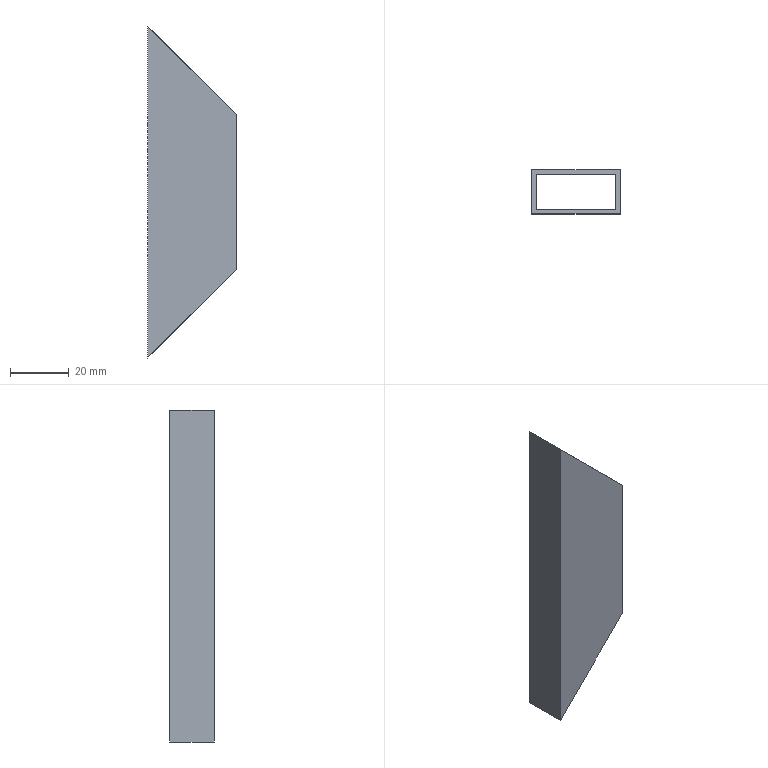Part | STEP file | Q7C0110 | 1 solid | 10 faces | box 30 x 15 x 113 mm | volume 10458 mm3 | plane 10
STEP:
#1=CARTESIAN_POINT('',(0.,0.,0.));
#2=DIRECTION('',(0.,0.,1.));
#3=DIRECTION('',(1.,0.,0.));
#4=AXIS2_PLACEMENT_3D('',#1,#2,#3);
#5=CARTESIAN_POINT('',(15.,7.5,83.));
#6=VERTEX_POINT('',#5);
#7=CARTESIAN_POINT('',(15.,7.5,30.));
#8=VERTEX_POINT('',#7);
#9=CARTESIAN_POINT('',(15.,7.5,150.));
#10=DIRECTION('',(0.,0.,-1.));
#11=VECTOR('',#10,1.);
#12=LINE('',#9,#11);
#13=CARTESIAN_POINT('',(15.,7.5,150.));
#14=DIRECTION('',(-1.,0.,0.));
#15=DIRECTION('',(0.,0.,1.));
#16=AXIS2_PLACEMENT_3D('',#13,#14,#15);
#17=PLANE('',#16);
#18=CARTESIAN_POINT('',(0.,0.));
#19=DIRECTION('',(-1.,0.));
#20=VECTOR('',#19,1.);
#21=LINE('',#18,#20);
#22=(GEOMETRIC_REPRESENTATION_CONTEXT(2)PARAMETRIC_REPRESENTATION_CONTEXT()REPRESENTATION_CONTEXT('',''));
#23=DEFINITIONAL_REPRESENTATION('',(#21),#22);
#24=PCURVE('',#17,#23);
#25=CARTESIAN_POINT('',(-15.,7.5,150.));
#26=DIRECTION('',(0.,-1.,0.));
#27=DIRECTION('',(0.,0.,-1.));
#28=AXIS2_PLACEMENT_3D('',#25,#26,#27);
#29=PLANE('',#28);
#30=CARTESIAN_POINT('',(0.,30.));
#31=DIRECTION('',(1.,0.));
#32=VECTOR('',#31,1.);
#33=LINE('',#30,#32);
#34=(GEOMETRIC_REPRESENTATION_CONTEXT(2)PARAMETRIC_REPRESENTATION_CONTEXT()REPRESENTATION_CONTEXT('',''));
#35=DEFINITIONAL_REPRESENTATION('',(#33),#34);
#36=PCURVE('',#29,#35);
#37=SURFACE_CURVE('',#12,(#24,#36),.PCURVE_S1.);
#38=EDGE_CURVE('',#6,#8,#37,.T.);
#39=ORIENTED_EDGE('',*,*,#38,.F.);
#40=CARTESIAN_POINT('',(15.,-7.5,83.));
#41=VERTEX_POINT('',#40);
#42=CARTESIAN_POINT('',(15.,-7.5,83.));
#43=DIRECTION('',(0.,1.,0.));
#44=VECTOR('',#43,1.);
#45=LINE('',#42,#44);
#46=CARTESIAN_POINT('',(-67.,-15.));
#47=DIRECTION('',(0.,1.));
#48=VECTOR('',#47,1.);
#49=LINE('',#46,#48);
#50=(GEOMETRIC_REPRESENTATION_CONTEXT(2)PARAMETRIC_REPRESENTATION_CONTEXT()REPRESENTATION_CONTEXT('',''));
#51=DEFINITIONAL_REPRESENTATION('',(#49),#50);
#52=PCURVE('',#17,#51);
#53=CARTESIAN_POINT('',(15.,-7.5,83.));
#54=DIRECTION('',(-0.7071,0.,-0.7071));
#55=DIRECTION('',(-0.7071,0.,0.7071));
#56=AXIS2_PLACEMENT_3D('',#53,#54,#55);
#57=PLANE('',#56);
#58=CARTESIAN_POINT('',(0.,0.));
#59=DIRECTION('',(0.,1.));
#60=VECTOR('',#59,1.);
#61=LINE('',#58,#60);
#62=(GEOMETRIC_REPRESENTATION_CONTEXT(2)PARAMETRIC_REPRESENTATION_CONTEXT()REPRESENTATION_CONTEXT('',''));
#63=DEFINITIONAL_REPRESENTATION('',(#61),#62);
#64=PCURVE('',#57,#63);
#65=SURFACE_CURVE('',#45,(#52,#64),.PCURVE_S1.);
#66=EDGE_CURVE('',#41,#6,#65,.T.);
#67=ORIENTED_EDGE('',*,*,#66,.F.);
#68=CARTESIAN_POINT('',(15.,-7.5,30.));
#69=VERTEX_POINT('',#68);
#70=CARTESIAN_POINT('',(15.,-7.5,150.));
#71=DIRECTION('',(0.,0.,-1.));
#72=VECTOR('',#71,1.);
#73=LINE('',#70,#72);
#74=CARTESIAN_POINT('',(0.,-15.));
#75=DIRECTION('',(-1.,0.));
#76=VECTOR('',#75,1.);
#77=LINE('',#74,#76);
#78=(GEOMETRIC_REPRESENTATION_CONTEXT(2)PARAMETRIC_REPRESENTATION_CONTEXT()REPRESENTATION_CONTEXT('',''));
#79=DEFINITIONAL_REPRESENTATION('',(#77),#78);
#80=PCURVE('',#17,#79);
#81=CARTESIAN_POINT('',(-15.,-7.5,150.));
#82=DIRECTION('',(0.,1.,0.));
#83=DIRECTION('',(0.,0.,1.));
#84=AXIS2_PLACEMENT_3D('',#81,#82,#83);
#85=PLANE('',#84);
#86=CARTESIAN_POINT('',(0.,30.));
#87=DIRECTION('',(-1.,0.));
#88=VECTOR('',#87,1.);
#89=LINE('',#86,#88);
#90=(GEOMETRIC_REPRESENTATION_CONTEXT(2)PARAMETRIC_REPRESENTATION_CONTEXT()REPRESENTATION_CONTEXT('',''));
#91=DEFINITIONAL_REPRESENTATION('',(#89),#90);
#92=PCURVE('',#85,#91);
#93=SURFACE_CURVE('',#73,(#80,#92),.PCURVE_S1.);
#94=EDGE_CURVE('',#41,#69,#93,.T.);
#95=ORIENTED_EDGE('',*,*,#94,.T.);
#96=CARTESIAN_POINT('',(15.,-7.5,30.));
#97=DIRECTION('',(0.,1.,0.));
#98=VECTOR('',#97,1.);
#99=LINE('',#96,#98);
#100=CARTESIAN_POINT('',(-120.,-15.));
#101=DIRECTION('',(0.,1.));
#102=VECTOR('',#101,1.);
#103=LINE('',#100,#102);
#104=(GEOMETRIC_REPRESENTATION_CONTEXT(2)PARAMETRIC_REPRESENTATION_CONTEXT()REPRESENTATION_CONTEXT('',''));
#105=DEFINITIONAL_REPRESENTATION('',(#103),#104);
#106=PCURVE('',#17,#105);
#107=CARTESIAN_POINT('',(-15.,-7.5,0.));
#108=DIRECTION('',(-0.7071,0.,0.7071));
#109=DIRECTION('',(0.7071,0.,0.7071));
#110=AXIS2_PLACEMENT_3D('',#107,#108,#109);
#111=PLANE('',#110);
#112=CARTESIAN_POINT('',(42.426,0.));
#113=DIRECTION('',(0.,1.));
#114=VECTOR('',#113,1.);
#115=LINE('',#112,#114);
#116=(GEOMETRIC_REPRESENTATION_CONTEXT(2)PARAMETRIC_REPRESENTATION_CONTEXT()REPRESENTATION_CONTEXT('',''));
#117=DEFINITIONAL_REPRESENTATION('',(#115),#116);
#118=PCURVE('',#111,#117);
#119=SURFACE_CURVE('',#99,(#106,#118),.PCURVE_S1.);
#120=EDGE_CURVE('',#69,#8,#119,.T.);
#121=ORIENTED_EDGE('',*,*,#120,.T.);
#122=EDGE_LOOP('',(#39,#67,#95,#121));
#123=FACE_BOUND('',#122,.T.);
#124=ADVANCED_FACE('',(#123),#17,.F.);
#125=CARTESIAN_POINT('',(-15.,7.5,113.));
#126=VERTEX_POINT('',#125);
#127=CARTESIAN_POINT('',(-15.,7.5,0.));
#128=VERTEX_POINT('',#127);
#129=CARTESIAN_POINT('',(-15.,7.5,150.));
#130=DIRECTION('',(0.,0.,-1.));
#131=VECTOR('',#130,1.);
#132=LINE('',#129,#131);
#133=CARTESIAN_POINT('',(0.,0.));
#134=DIRECTION('',(1.,0.));
#135=VECTOR('',#134,1.);
#136=LINE('',#133,#135);
#137=(GEOMETRIC_REPRESENTATION_CONTEXT(2)PARAMETRIC_REPRESENTATION_CONTEXT()REPRESENTATION_CONTEXT('',''));
#138=DEFINITIONAL_REPRESENTATION('',(#136),#137);
#139=PCURVE('',#29,#138);
#140=CARTESIAN_POINT('',(-15.,7.5,150.));
#141=DIRECTION('',(1.,0.,0.));
#142=DIRECTION('',(0.,0.,-1.));
#143=AXIS2_PLACEMENT_3D('',#140,#141,#142);
#144=PLANE('',#143);
#145=CARTESIAN_POINT('',(0.,0.));
#146=DIRECTION('',(1.,0.));
#147=VECTOR('',#146,1.);
#148=LINE('',#145,#147);
#149=(GEOMETRIC_REPRESENTATION_CONTEXT(2)PARAMETRIC_REPRESENTATION_CONTEXT()REPRESENTATION_CONTEXT('',''));
#150=DEFINITIONAL_REPRESENTATION('',(#148),#149);
#151=PCURVE('',#144,#150);
#152=SURFACE_CURVE('',#132,(#139,#151),.PCURVE_S1.);
#153=EDGE_CURVE('',#126,#128,#152,.T.);
#154=ORIENTED_EDGE('',*,*,#153,.F.);
#155=CARTESIAN_POINT('',(15.,7.5,83.));
#156=DIRECTION('',(-0.7071,0.,0.7071));
#157=VECTOR('',#156,1.);
#158=LINE('',#155,#157);
#159=CARTESIAN_POINT('',(67.,30.));
#160=DIRECTION('',(-0.7071,-0.7071));
#161=VECTOR('',#160,1.);
#162=LINE('',#159,#161);
#163=(GEOMETRIC_REPRESENTATION_CONTEXT(2)PARAMETRIC_REPRESENTATION_CONTEXT()REPRESENTATION_CONTEXT('',''));
#164=DEFINITIONAL_REPRESENTATION('',(#162),#163);
#165=PCURVE('',#29,#164);
#166=CARTESIAN_POINT('',(0.,15.));
#167=DIRECTION('',(1.,0.));
#168=VECTOR('',#167,1.);
#169=LINE('',#166,#168);
#170=(GEOMETRIC_REPRESENTATION_CONTEXT(2)PARAMETRIC_REPRESENTATION_CONTEXT()REPRESENTATION_CONTEXT('',''));
#171=DEFINITIONAL_REPRESENTATION('',(#169),#170);
#172=PCURVE('',#57,#171);
#173=SURFACE_CURVE('',#158,(#165,#172),.PCURVE_S1.);
#174=EDGE_CURVE('',#6,#126,#173,.T.);
#175=ORIENTED_EDGE('',*,*,#174,.F.);
#176=ORIENTED_EDGE('',*,*,#38,.T.);
#177=CARTESIAN_POINT('',(-15.,7.5,0.));
#178=DIRECTION('',(0.7071,0.,0.7071));
#179=VECTOR('',#178,1.);
#180=LINE('',#177,#179);
#181=CARTESIAN_POINT('',(150.,0.));
#182=DIRECTION('',(-0.7071,0.7071));
#183=VECTOR('',#182,1.);
#184=LINE('',#181,#183);
#185=(GEOMETRIC_REPRESENTATION_CONTEXT(2)PARAMETRIC_REPRESENTATION_CONTEXT()REPRESENTATION_CONTEXT('',''));
#186=DEFINITIONAL_REPRESENTATION('',(#184),#185);
#187=PCURVE('',#29,#186);
#188=CARTESIAN_POINT('',(0.,15.));
#189=DIRECTION('',(1.,0.));
#190=VECTOR('',#189,1.);
#191=LINE('',#188,#190);
#192=(GEOMETRIC_REPRESENTATION_CONTEXT(2)PARAMETRIC_REPRESENTATION_CONTEXT()REPRESENTATION_CONTEXT('',''));
#193=DEFINITIONAL_REPRESENTATION('',(#191),#192);
#194=PCURVE('',#111,#193);
#195=SURFACE_CURVE('',#180,(#187,#194),.PCURVE_S1.);
#196=EDGE_CURVE('',#128,#8,#195,.T.);
#197=ORIENTED_EDGE('',*,*,#196,.F.);
#198=EDGE_LOOP('',(#154,#175,#176,#197));
#199=FACE_BOUND('',#198,.T.);
#200=ADVANCED_FACE('',(#199),#29,.F.);
#201=CARTESIAN_POINT('',(-15.,-7.5,113.));
#202=VERTEX_POINT('',#201);
#203=CARTESIAN_POINT('',(-15.,-7.5,0.));
#204=VERTEX_POINT('',#203);
#205=CARTESIAN_POINT('',(-15.,-7.5,150.));
#206=DIRECTION('',(0.,0.,-1.));
#207=VECTOR('',#206,1.);
#208=LINE('',#205,#207);
#209=CARTESIAN_POINT('',(0.,-15.));
#210=DIRECTION('',(1.,0.));
#211=VECTOR('',#210,1.);
#212=LINE('',#209,#211);
#213=(GEOMETRIC_REPRESENTATION_CONTEXT(2)PARAMETRIC_REPRESENTATION_CONTEXT()REPRESENTATION_CONTEXT('',''));
#214=DEFINITIONAL_REPRESENTATION('',(#212),#213);
#215=PCURVE('',#144,#214);
#216=CARTESIAN_POINT('',(0.,0.));
#217=DIRECTION('',(-1.,0.));
#218=VECTOR('',#217,1.);
#219=LINE('',#216,#218);
#220=(GEOMETRIC_REPRESENTATION_CONTEXT(2)PARAMETRIC_REPRESENTATION_CONTEXT()REPRESENTATION_CONTEXT('',''));
#221=DEFINITIONAL_REPRESENTATION('',(#219),#220);
#222=PCURVE('',#85,#221);
#223=SURFACE_CURVE('',#208,(#215,#222),.PCURVE_S1.);
#224=EDGE_CURVE('',#202,#204,#223,.T.);
#225=ORIENTED_EDGE('',*,*,#224,.F.);
#226=CARTESIAN_POINT('',(-15.,7.5,113.));
#227=DIRECTION('',(0.,1.,0.));
#228=VECTOR('',#227,1.);
#229=LINE('',#226,#228);
#230=CARTESIAN_POINT('',(37.,0.));
#231=DIRECTION('',(0.,1.));
#232=VECTOR('',#231,1.);
#233=LINE('',#230,#232);
#234=(GEOMETRIC_REPRESENTATION_CONTEXT(2)PARAMETRIC_REPRESENTATION_CONTEXT()REPRESENTATION_CONTEXT('',''));
#235=DEFINITIONAL_REPRESENTATION('',(#233),#234);
#236=PCURVE('',#144,#235);
#237=CARTESIAN_POINT('',(42.426,15.));
#238=DIRECTION('',(0.,1.));
#239=VECTOR('',#238,1.);
#240=LINE('',#237,#239);
#241=(GEOMETRIC_REPRESENTATION_CONTEXT(2)PARAMETRIC_REPRESENTATION_CONTEXT()REPRESENTATION_CONTEXT('',''));
#242=DEFINITIONAL_REPRESENTATION('',(#240),#241);
#243=PCURVE('',#57,#242);
#244=SURFACE_CURVE('',#229,(#236,#243),.PCURVE_S1.);
#245=EDGE_CURVE('',#202,#126,#244,.T.);
#246=ORIENTED_EDGE('',*,*,#245,.T.);
#247=ORIENTED_EDGE('',*,*,#153,.T.);
#248=CARTESIAN_POINT('',(-15.,7.5,0.));
#249=DIRECTION('',(0.,-1.,0.));
#250=VECTOR('',#249,1.);
#251=LINE('',#248,#250);
#252=CARTESIAN_POINT('',(150.,0.));
#253=DIRECTION('',(0.,-1.));
#254=VECTOR('',#253,1.);
#255=LINE('',#252,#254);
#256=(GEOMETRIC_REPRESENTATION_CONTEXT(2)PARAMETRIC_REPRESENTATION_CONTEXT()REPRESENTATION_CONTEXT('',''));
#257=DEFINITIONAL_REPRESENTATION('',(#255),#256);
#258=PCURVE('',#144,#257);
#259=CARTESIAN_POINT('',(0.,15.));
#260=DIRECTION('',(0.,-1.));
#261=VECTOR('',#260,1.);
#262=LINE('',#259,#261);
#263=(GEOMETRIC_REPRESENTATION_CONTEXT(2)PARAMETRIC_REPRESENTATION_CONTEXT()REPRESENTATION_CONTEXT('',''));
#264=DEFINITIONAL_REPRESENTATION('',(#262),#263);
#265=PCURVE('',#111,#264);
#266=SURFACE_CURVE('',#251,(#258,#265),.PCURVE_S1.);
#267=EDGE_CURVE('',#128,#204,#266,.T.);
#268=ORIENTED_EDGE('',*,*,#267,.T.);
#269=EDGE_LOOP('',(#225,#246,#247,#268));
#270=FACE_BOUND('',#269,.T.);
#271=ADVANCED_FACE('',(#270),#144,.F.);
#272=ORIENTED_EDGE('',*,*,#94,.F.);
#273=CARTESIAN_POINT('',(15.,-7.5,83.));
#274=DIRECTION('',(-0.7071,0.,0.7071));
#275=VECTOR('',#274,1.);
#276=LINE('',#273,#275);
#277=CARTESIAN_POINT('',(-67.,30.));
#278=DIRECTION('',(0.7071,-0.7071));
#279=VECTOR('',#278,1.);
#280=LINE('',#277,#279);
#281=(GEOMETRIC_REPRESENTATION_CONTEXT(2)PARAMETRIC_REPRESENTATION_CONTEXT()REPRESENTATION_CONTEXT('',''));
#282=DEFINITIONAL_REPRESENTATION('',(#280),#281);
#283=PCURVE('',#85,#282);
#284=CARTESIAN_POINT('',(0.,0.));
#285=DIRECTION('',(1.,0.));
#286=VECTOR('',#285,1.);
#287=LINE('',#284,#286);
#288=(GEOMETRIC_REPRESENTATION_CONTEXT(2)PARAMETRIC_REPRESENTATION_CONTEXT()REPRESENTATION_CONTEXT('',''));
#289=DEFINITIONAL_REPRESENTATION('',(#287),#288);
#290=PCURVE('',#57,#289);
#291=SURFACE_CURVE('',#276,(#283,#290),.PCURVE_S1.);
#292=EDGE_CURVE('',#41,#202,#291,.T.);
#293=ORIENTED_EDGE('',*,*,#292,.T.);
#294=ORIENTED_EDGE('',*,*,#224,.T.);
#295=CARTESIAN_POINT('',(-15.,-7.5,0.));
#296=DIRECTION('',(0.7071,0.,0.7071));
#297=VECTOR('',#296,1.);
#298=LINE('',#295,#297);
#299=CARTESIAN_POINT('',(-150.,0.));
#300=DIRECTION('',(0.7071,0.7071));
#301=VECTOR('',#300,1.);
#302=LINE('',#299,#301);
#303=(GEOMETRIC_REPRESENTATION_CONTEXT(2)PARAMETRIC_REPRESENTATION_CONTEXT()REPRESENTATION_CONTEXT('',''));
#304=DEFINITIONAL_REPRESENTATION('',(#302),#303);
#305=PCURVE('',#85,#304);
#306=CARTESIAN_POINT('',(0.,0.));
#307=DIRECTION('',(1.,0.));
#308=VECTOR('',#307,1.);
#309=LINE('',#306,#308);
#310=(GEOMETRIC_REPRESENTATION_CONTEXT(2)PARAMETRIC_REPRESENTATION_CONTEXT()REPRESENTATION_CONTEXT('',''));
#311=DEFINITIONAL_REPRESENTATION('',(#309),#310);
#312=PCURVE('',#111,#311);
#313=SURFACE_CURVE('',#298,(#305,#312),.PCURVE_S1.);
#314=EDGE_CURVE('',#204,#69,#313,.T.);
#315=ORIENTED_EDGE('',*,*,#314,.T.);
#316=EDGE_LOOP('',(#272,#293,#294,#315));
#317=FACE_BOUND('',#316,.T.);
#318=ADVANCED_FACE('',(#317),#85,.F.);
#319=CARTESIAN_POINT('',(-13.5,-6.,111.5));
#320=VERTEX_POINT('',#319);
#321=CARTESIAN_POINT('',(-13.5,6.,111.5));
#322=VERTEX_POINT('',#321);
#323=CARTESIAN_POINT('',(-13.5,6.,111.5));
#324=DIRECTION('',(0.,1.,0.));
#325=VECTOR('',#324,1.);
#326=LINE('',#323,#325);
#327=CARTESIAN_POINT('',(-13.5,6.,150.));
#328=DIRECTION('',(1.,0.,0.));
#329=DIRECTION('',(0.,1.,0.));
#330=AXIS2_PLACEMENT_3D('',#327,#328,#329);
#331=PLANE('',#330);
#332=CARTESIAN_POINT('',(0.,-38.5));
#333=DIRECTION('',(1.,0.));
#334=VECTOR('',#333,1.);
#335=LINE('',#332,#334);
#336=(GEOMETRIC_REPRESENTATION_CONTEXT(2)PARAMETRIC_REPRESENTATION_CONTEXT()REPRESENTATION_CONTEXT('',''));
#337=DEFINITIONAL_REPRESENTATION('',(#335),#336);
#338=PCURVE('',#331,#337);
#339=CARTESIAN_POINT('',(40.305,13.5));
#340=DIRECTION('',(0.,1.));
#341=VECTOR('',#340,1.);
#342=LINE('',#339,#341);
#343=(GEOMETRIC_REPRESENTATION_CONTEXT(2)PARAMETRIC_REPRESENTATION_CONTEXT()REPRESENTATION_CONTEXT('',''));
#344=DEFINITIONAL_REPRESENTATION('',(#342),#343);
#345=PCURVE('',#57,#344);
#346=SURFACE_CURVE('',#326,(#338,#345),.PCURVE_S1.);
#347=EDGE_CURVE('',#320,#322,#346,.T.);
#348=ORIENTED_EDGE('',*,*,#347,.F.);
#349=CARTESIAN_POINT('',(-13.5,-6.,1.5));
#350=VERTEX_POINT('',#349);
#351=CARTESIAN_POINT('',(-13.5,-6.,150.));
#352=DIRECTION('',(0.,0.,-1.));
#353=VECTOR('',#352,1.);
#354=LINE('',#351,#353);
#355=CARTESIAN_POINT('',(-12.,0.));
#356=DIRECTION('',(0.,-1.));
#357=VECTOR('',#356,1.);
#358=LINE('',#355,#357);
#359=(GEOMETRIC_REPRESENTATION_CONTEXT(2)PARAMETRIC_REPRESENTATION_CONTEXT()REPRESENTATION_CONTEXT('',''));
#360=DEFINITIONAL_REPRESENTATION('',(#358),#359);
#361=PCURVE('',#331,#360);
#362=CARTESIAN_POINT('',(-13.5,-6.,150.));
#363=DIRECTION('',(0.,1.,0.));
#364=DIRECTION('',(-1.,0.,0.));
#365=AXIS2_PLACEMENT_3D('',#362,#363,#364);
#366=PLANE('',#365);
#367=CARTESIAN_POINT('',(0.,0.));
#368=DIRECTION('',(0.,-1.));
#369=VECTOR('',#368,1.);
#370=LINE('',#367,#369);
#371=(GEOMETRIC_REPRESENTATION_CONTEXT(2)PARAMETRIC_REPRESENTATION_CONTEXT()REPRESENTATION_CONTEXT('',''));
#372=DEFINITIONAL_REPRESENTATION('',(#370),#371);
#373=PCURVE('',#366,#372);
#374=SURFACE_CURVE('',#354,(#361,#373),.PCURVE_S1.);
#375=EDGE_CURVE('',#320,#350,#374,.T.);
#376=ORIENTED_EDGE('',*,*,#375,.T.);
#377=CARTESIAN_POINT('',(-13.5,6.,1.5));
#378=VERTEX_POINT('',#377);
#379=CARTESIAN_POINT('',(-13.5,6.,1.5));
#380=DIRECTION('',(0.,-1.,0.));
#381=VECTOR('',#380,1.);
#382=LINE('',#379,#381);
#383=CARTESIAN_POINT('',(0.,-148.5));
#384=DIRECTION('',(-1.,0.));
#385=VECTOR('',#384,1.);
#386=LINE('',#383,#385);
#387=(GEOMETRIC_REPRESENTATION_CONTEXT(2)PARAMETRIC_REPRESENTATION_CONTEXT()REPRESENTATION_CONTEXT('',''));
#388=DEFINITIONAL_REPRESENTATION('',(#386),#387);
#389=PCURVE('',#331,#388);
#390=CARTESIAN_POINT('',(2.121,13.5));
#391=DIRECTION('',(0.,-1.));
#392=VECTOR('',#391,1.);
#393=LINE('',#390,#392);
#394=(GEOMETRIC_REPRESENTATION_CONTEXT(2)PARAMETRIC_REPRESENTATION_CONTEXT()REPRESENTATION_CONTEXT('',''));
#395=DEFINITIONAL_REPRESENTATION('',(#393),#394);
#396=PCURVE('',#111,#395);
#397=SURFACE_CURVE('',#382,(#389,#396),.PCURVE_S1.);
#398=EDGE_CURVE('',#378,#350,#397,.T.);
#399=ORIENTED_EDGE('',*,*,#398,.F.);
#400=CARTESIAN_POINT('',(-13.5,6.,150.));
#401=DIRECTION('',(0.,0.,-1.));
#402=VECTOR('',#401,1.);
#403=LINE('',#400,#402);
#404=CARTESIAN_POINT('',(0.,0.));
#405=DIRECTION('',(0.,-1.));
#406=VECTOR('',#405,1.);
#407=LINE('',#404,#406);
#408=(GEOMETRIC_REPRESENTATION_CONTEXT(2)PARAMETRIC_REPRESENTATION_CONTEXT()REPRESENTATION_CONTEXT('',''));
#409=DEFINITIONAL_REPRESENTATION('',(#407),#408);
#410=PCURVE('',#331,#409);
#411=CARTESIAN_POINT('',(-13.5,6.,150.));
#412=DIRECTION('',(0.,-1.,0.));
#413=DIRECTION('',(0.,0.,-1.));
#414=AXIS2_PLACEMENT_3D('',#411,#412,#413);
#415=PLANE('',#414);
#416=CARTESIAN_POINT('',(0.,0.));
#417=DIRECTION('',(1.,0.));
#418=VECTOR('',#417,1.);
#419=LINE('',#416,#418);
#420=(GEOMETRIC_REPRESENTATION_CONTEXT(2)PARAMETRIC_REPRESENTATION_CONTEXT()REPRESENTATION_CONTEXT('',''));
#421=DEFINITIONAL_REPRESENTATION('',(#419),#420);
#422=PCURVE('',#415,#421);
#423=SURFACE_CURVE('',#403,(#410,#422),.PCURVE_S1.);
#424=EDGE_CURVE('',#322,#378,#423,.T.);
#425=ORIENTED_EDGE('',*,*,#424,.F.);
#426=EDGE_LOOP('',(#348,#376,#399,#425));
#427=FACE_BOUND('',#426,.T.);
#428=ADVANCED_FACE('',(#427),#331,.T.);
#429=CARTESIAN_POINT('',(13.5,-6.,84.5));
#430=VERTEX_POINT('',#429);
#431=CARTESIAN_POINT('',(-32.75,-6.,130.75));
#432=DIRECTION('',(-0.7071,0.,0.7071));
#433=VECTOR('',#432,1.);
#434=LINE('',#431,#433);
#435=CARTESIAN_POINT('',(19.25,-19.25));
#436=DIRECTION('',(0.7071,0.7071));
#437=VECTOR('',#436,1.);
#438=LINE('',#435,#437);
#439=(GEOMETRIC_REPRESENTATION_CONTEXT(2)PARAMETRIC_REPRESENTATION_CONTEXT()REPRESENTATION_CONTEXT('',''));
#440=DEFINITIONAL_REPRESENTATION('',(#438),#439);
#441=PCURVE('',#366,#440);
#442=CARTESIAN_POINT('',(67.529,1.5));
#443=DIRECTION('',(1.,0.));
#444=VECTOR('',#443,1.);
#445=LINE('',#442,#444);
#446=(GEOMETRIC_REPRESENTATION_CONTEXT(2)PARAMETRIC_REPRESENTATION_CONTEXT()REPRESENTATION_CONTEXT('',''));
#447=DEFINITIONAL_REPRESENTATION('',(#445),#446);
#448=PCURVE('',#57,#447);
#449=SURFACE_CURVE('',#434,(#441,#448),.PCURVE_S1.);
#450=EDGE_CURVE('',#430,#320,#449,.T.);
#451=ORIENTED_EDGE('',*,*,#450,.F.);
#452=CARTESIAN_POINT('',(13.5,-6.,28.5));
#453=VERTEX_POINT('',#452);
#454=CARTESIAN_POINT('',(13.5,-6.,150.));
#455=DIRECTION('',(0.,0.,-1.));
#456=VECTOR('',#455,1.);
#457=LINE('',#454,#456);
#458=CARTESIAN_POINT('',(-27.,0.));
#459=DIRECTION('',(0.,-1.));
#460=VECTOR('',#459,1.);
#461=LINE('',#458,#460);
#462=(GEOMETRIC_REPRESENTATION_CONTEXT(2)PARAMETRIC_REPRESENTATION_CONTEXT()REPRESENTATION_CONTEXT('',''));
#463=DEFINITIONAL_REPRESENTATION('',(#461),#462);
#464=PCURVE('',#366,#463);
#465=CARTESIAN_POINT('',(13.5,6.,150.));
#466=DIRECTION('',(-1.,0.,0.));
#467=DIRECTION('',(0.,-1.,0.));
#468=AXIS2_PLACEMENT_3D('',#465,#466,#467);
#469=PLANE('',#468);
#470=CARTESIAN_POINT('',(12.,0.));
#471=DIRECTION('',(0.,-1.));
#472=VECTOR('',#471,1.);
#473=LINE('',#470,#472);
#474=(GEOMETRIC_REPRESENTATION_CONTEXT(2)PARAMETRIC_REPRESENTATION_CONTEXT()REPRESENTATION_CONTEXT('',''));
#475=DEFINITIONAL_REPRESENTATION('',(#473),#474);
#476=PCURVE('',#469,#475);
#477=SURFACE_CURVE('',#457,(#464,#476),.PCURVE_S1.);
#478=EDGE_CURVE('',#430,#453,#477,.T.);
#479=ORIENTED_EDGE('',*,*,#478,.T.);
#480=CARTESIAN_POINT('',(60.75,-6.,75.75));
#481=DIRECTION('',(0.7071,0.,0.7071));
#482=VECTOR('',#481,1.);
#483=LINE('',#480,#482);
#484=CARTESIAN_POINT('',(-74.25,-74.25));
#485=DIRECTION('',(-0.7071,0.7071));
#486=VECTOR('',#485,1.);
#487=LINE('',#484,#486);
#488=(GEOMETRIC_REPRESENTATION_CONTEXT(2)PARAMETRIC_REPRESENTATION_CONTEXT()REPRESENTATION_CONTEXT('',''));
#489=DEFINITIONAL_REPRESENTATION('',(#487),#488);
#490=PCURVE('',#366,#489);
#491=CARTESIAN_POINT('',(107.127,1.5));
#492=DIRECTION('',(1.,0.));
#493=VECTOR('',#492,1.);
#494=LINE('',#491,#493);
#495=(GEOMETRIC_REPRESENTATION_CONTEXT(2)PARAMETRIC_REPRESENTATION_CONTEXT()REPRESENTATION_CONTEXT('',''));
#496=DEFINITIONAL_REPRESENTATION('',(#494),#495);
#497=PCURVE('',#111,#496);
#498=SURFACE_CURVE('',#483,(#490,#497),.PCURVE_S1.);
#499=EDGE_CURVE('',#350,#453,#498,.T.);
#500=ORIENTED_EDGE('',*,*,#499,.F.);
#501=ORIENTED_EDGE('',*,*,#375,.F.);
#502=EDGE_LOOP('',(#451,#479,#500,#501));
#503=FACE_BOUND('',#502,.T.);
#504=ADVANCED_FACE('',(#503),#366,.T.);
#505=CARTESIAN_POINT('',(13.5,6.,84.5));
#506=VERTEX_POINT('',#505);
#507=CARTESIAN_POINT('',(13.5,6.,84.5));
#508=DIRECTION('',(0.,-1.,0.));
#509=VECTOR('',#508,1.);
#510=LINE('',#507,#509);
#511=CARTESIAN_POINT('',(0.,-65.5));
#512=DIRECTION('',(1.,0.));
#513=VECTOR('',#512,1.);
#514=LINE('',#511,#513);
#515=(GEOMETRIC_REPRESENTATION_CONTEXT(2)PARAMETRIC_REPRESENTATION_CONTEXT()REPRESENTATION_CONTEXT('',''));
#516=DEFINITIONAL_REPRESENTATION('',(#514),#515);
#517=PCURVE('',#469,#516);
#518=CARTESIAN_POINT('',(2.121,13.5));
#519=DIRECTION('',(0.,-1.));
#520=VECTOR('',#519,1.);
#521=LINE('',#518,#520);
#522=(GEOMETRIC_REPRESENTATION_CONTEXT(2)PARAMETRIC_REPRESENTATION_CONTEXT()REPRESENTATION_CONTEXT('',''));
#523=DEFINITIONAL_REPRESENTATION('',(#521),#522);
#524=PCURVE('',#57,#523);
#525=SURFACE_CURVE('',#510,(#517,#524),.PCURVE_S1.);
#526=EDGE_CURVE('',#506,#430,#525,.T.);
#527=ORIENTED_EDGE('',*,*,#526,.F.);
#528=CARTESIAN_POINT('',(13.5,6.,28.5));
#529=VERTEX_POINT('',#528);
#530=CARTESIAN_POINT('',(13.5,6.,150.));
#531=DIRECTION('',(0.,0.,-1.));
#532=VECTOR('',#531,1.);
#533=LINE('',#530,#532);
#534=CARTESIAN_POINT('',(0.,0.));
#535=DIRECTION('',(0.,-1.));
#536=VECTOR('',#535,1.);
#537=LINE('',#534,#536);
#538=(GEOMETRIC_REPRESENTATION_CONTEXT(2)PARAMETRIC_REPRESENTATION_CONTEXT()REPRESENTATION_CONTEXT('',''));
#539=DEFINITIONAL_REPRESENTATION('',(#537),#538);
#540=PCURVE('',#469,#539);
#541=CARTESIAN_POINT('',(0.,27.));
#542=DIRECTION('',(1.,0.));
#543=VECTOR('',#542,1.);
#544=LINE('',#541,#543);
#545=(GEOMETRIC_REPRESENTATION_CONTEXT(2)PARAMETRIC_REPRESENTATION_CONTEXT()REPRESENTATION_CONTEXT('',''));
#546=DEFINITIONAL_REPRESENTATION('',(#544),#545);
#547=PCURVE('',#415,#546);
#548=SURFACE_CURVE('',#533,(#540,#547),.PCURVE_S1.);
#549=EDGE_CURVE('',#506,#529,#548,.T.);
#550=ORIENTED_EDGE('',*,*,#549,.T.);
#551=CARTESIAN_POINT('',(13.5,6.,28.5));
#552=DIRECTION('',(0.,1.,0.));
#553=VECTOR('',#552,1.);
#554=LINE('',#551,#553);
#555=CARTESIAN_POINT('',(0.,-121.5));
#556=DIRECTION('',(-1.,0.));
#557=VECTOR('',#556,1.);
#558=LINE('',#555,#557);
#559=(GEOMETRIC_REPRESENTATION_CONTEXT(2)PARAMETRIC_REPRESENTATION_CONTEXT()REPRESENTATION_CONTEXT('',''));
#560=DEFINITIONAL_REPRESENTATION('',(#558),#559);
#561=PCURVE('',#469,#560);
#562=CARTESIAN_POINT('',(40.305,13.5));
#563=DIRECTION('',(0.,1.));
#564=VECTOR('',#563,1.);
#565=LINE('',#562,#564);
#566=(GEOMETRIC_REPRESENTATION_CONTEXT(2)PARAMETRIC_REPRESENTATION_CONTEXT()REPRESENTATION_CONTEXT('',''));
#567=DEFINITIONAL_REPRESENTATION('',(#565),#566);
#568=PCURVE('',#111,#567);
#569=SURFACE_CURVE('',#554,(#561,#568),.PCURVE_S1.);
#570=EDGE_CURVE('',#453,#529,#569,.T.);
#571=ORIENTED_EDGE('',*,*,#570,.F.);
#572=ORIENTED_EDGE('',*,*,#478,.F.);
#573=EDGE_LOOP('',(#527,#550,#571,#572));
#574=FACE_BOUND('',#573,.T.);
#575=ADVANCED_FACE('',(#574),#469,.T.);
#576=CARTESIAN_POINT('',(-32.75,6.,130.75));
#577=DIRECTION('',(0.7071,0.,-0.7071));
#578=VECTOR('',#577,1.);
#579=LINE('',#576,#578);
#580=CARTESIAN_POINT('',(19.25,-19.25));
#581=DIRECTION('',(0.7071,0.7071));
#582=VECTOR('',#581,1.);
#583=LINE('',#580,#582);
#584=(GEOMETRIC_REPRESENTATION_CONTEXT(2)PARAMETRIC_REPRESENTATION_CONTEXT()REPRESENTATION_CONTEXT('',''));
#585=DEFINITIONAL_REPRESENTATION('',(#583),#584);
#586=PCURVE('',#415,#585);
#587=CARTESIAN_POINT('',(67.529,13.5));
#588=DIRECTION('',(-1.,0.));
#589=VECTOR('',#588,1.);
#590=LINE('',#587,#589);
#591=(GEOMETRIC_REPRESENTATION_CONTEXT(2)PARAMETRIC_REPRESENTATION_CONTEXT()REPRESENTATION_CONTEXT('',''));
#592=DEFINITIONAL_REPRESENTATION('',(#590),#591);
#593=PCURVE('',#57,#592);
#594=SURFACE_CURVE('',#579,(#586,#593),.PCURVE_S1.);
#595=EDGE_CURVE('',#322,#506,#594,.T.);
#596=ORIENTED_EDGE('',*,*,#595,.F.);
#597=ORIENTED_EDGE('',*,*,#424,.T.);
#598=CARTESIAN_POINT('',(60.75,6.,75.75));
#599=DIRECTION('',(-0.7071,0.,-0.7071));
#600=VECTOR('',#599,1.);
#601=LINE('',#598,#600);
#602=CARTESIAN_POINT('',(74.25,74.25));
#603=DIRECTION('',(0.7071,-0.7071));
#604=VECTOR('',#603,1.);
#605=LINE('',#602,#604);
#606=(GEOMETRIC_REPRESENTATION_CONTEXT(2)PARAMETRIC_REPRESENTATION_CONTEXT()REPRESENTATION_CONTEXT('',''));
#607=DEFINITIONAL_REPRESENTATION('',(#605),#606);
#608=PCURVE('',#415,#607);
#609=CARTESIAN_POINT('',(107.127,13.5));
#610=DIRECTION('',(-1.,0.));
#611=VECTOR('',#610,1.);
#612=LINE('',#609,#611);
#613=(GEOMETRIC_REPRESENTATION_CONTEXT(2)PARAMETRIC_REPRESENTATION_CONTEXT()REPRESENTATION_CONTEXT('',''));
#614=DEFINITIONAL_REPRESENTATION('',(#612),#613);
#615=PCURVE('',#111,#614);
#616=SURFACE_CURVE('',#601,(#608,#615),.PCURVE_S1.);
#617=EDGE_CURVE('',#529,#378,#616,.T.);
#618=ORIENTED_EDGE('',*,*,#617,.F.);
#619=ORIENTED_EDGE('',*,*,#549,.F.);
#620=EDGE_LOOP('',(#596,#597,#618,#619));
#621=FACE_BOUND('',#620,.T.);
#622=ADVANCED_FACE('',(#621),#415,.T.);
#623=ORIENTED_EDGE('',*,*,#398,.T.);
#624=ORIENTED_EDGE('',*,*,#499,.T.);
#625=ORIENTED_EDGE('',*,*,#570,.T.);
#626=ORIENTED_EDGE('',*,*,#617,.T.);
#627=EDGE_LOOP('',(#623,#624,#625,#626));
#628=FACE_BOUND('',#627,.T.);
#629=ORIENTED_EDGE('',*,*,#196,.T.);
#630=ORIENTED_EDGE('',*,*,#120,.F.);
#631=ORIENTED_EDGE('',*,*,#314,.F.);
#632=ORIENTED_EDGE('',*,*,#267,.F.);
#633=EDGE_LOOP('',(#629,#630,#631,#632));
#634=FACE_BOUND('',#633,.T.);
#635=ADVANCED_FACE('',(#628,#634),#111,.F.);
#636=ORIENTED_EDGE('',*,*,#347,.T.);
#637=ORIENTED_EDGE('',*,*,#595,.T.);
#638=ORIENTED_EDGE('',*,*,#526,.T.);
#639=ORIENTED_EDGE('',*,*,#450,.T.);
#640=EDGE_LOOP('',(#636,#637,#638,#639));
#641=FACE_BOUND('',#640,.T.);
#642=ORIENTED_EDGE('',*,*,#292,.F.);
#643=ORIENTED_EDGE('',*,*,#66,.T.);
#644=ORIENTED_EDGE('',*,*,#174,.T.);
#645=ORIENTED_EDGE('',*,*,#245,.F.);
#646=EDGE_LOOP('',(#642,#643,#644,#645));
#647=FACE_BOUND('',#646,.T.);
#648=ADVANCED_FACE('',(#641,#647),#57,.F.);
#649=CLOSED_SHELL('',(#124,#200,#271,#318,#428,#504,#575,#622,#635,#648));
#650=MANIFOLD_SOLID_BREP('',#649);
#651=(LENGTH_UNIT()NAMED_UNIT(*)SI_UNIT(.MILLI.,.METRE.));
#652=UNCERTAINTY_MEASURE_WITH_UNIT(LENGTH_MEASURE(0.0000001),#651,'','');
#653=(NAMED_UNIT(*)PLANE_ANGLE_UNIT()SI_UNIT($,.RADIAN.));
#654=(NAMED_UNIT(*)SI_UNIT($,.STERADIAN.)SOLID_ANGLE_UNIT());
#655=(GEOMETRIC_REPRESENTATION_CONTEXT(3)GLOBAL_UNCERTAINTY_ASSIGNED_CONTEXT((#652))GLOBAL_UNIT_ASSIGNED_CONTEXT((#651,#653,#654))REPRESENTATION_CONTEXT('',''));
#656=ADVANCED_BREP_SHAPE_REPRESENTATION('',(#4,#650),#655);